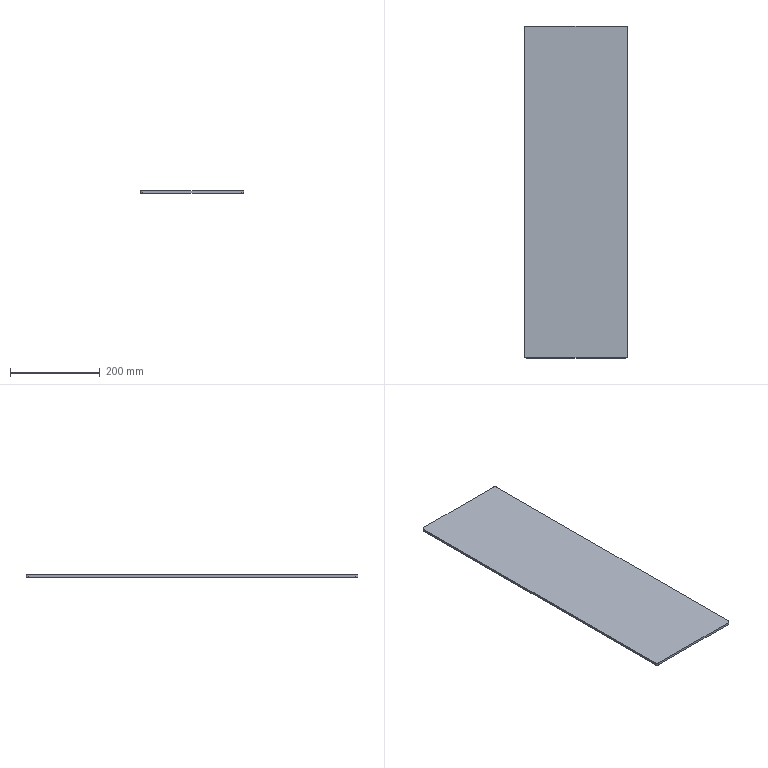Part | STEP file | 001-002-Face Plate-3 | 1 solid | 10 faces | box 230 x 740 x 5 mm | volume 850893 mm3 | plane 6 | cylinder 4 | commonest cylinder face diameters 10 x4
STEP:
#1=CARTESIAN_POINT('',(0.,0.,0.));
#2=DIRECTION('',(0.,0.,1.));
#3=DIRECTION('',(1.,0.,0.));
#4=AXIS2_PLACEMENT_3D('',#1,#2,#3);
#5=CARTESIAN_POINT('',(115.,-365.,0.));
#6=VERTEX_POINT('',#5);
#7=CARTESIAN_POINT('',(115.,365.,0.));
#8=VERTEX_POINT('',#7);
#9=CARTESIAN_POINT('',(115.,-370.,0.));
#10=DIRECTION('',(0.,1.,0.));
#11=VECTOR('',#10,1.);
#12=LINE('',#9,#11);
#13=CARTESIAN_POINT('',(115.,-370.,5.));
#14=DIRECTION('',(-1.,0.,0.));
#15=DIRECTION('',(0.,0.,1.));
#16=AXIS2_PLACEMENT_3D('',#13,#14,#15);
#17=PLANE('',#16);
#18=CARTESIAN_POINT('',(-5.,0.));
#19=DIRECTION('',(0.,1.));
#20=VECTOR('',#19,1.);
#21=LINE('',#18,#20);
#22=(GEOMETRIC_REPRESENTATION_CONTEXT(2)PARAMETRIC_REPRESENTATION_CONTEXT()REPRESENTATION_CONTEXT('',''));
#23=DEFINITIONAL_REPRESENTATION('',(#21),#22);
#24=PCURVE('',#17,#23);
#25=CARTESIAN_POINT('',(0.,0.,0.));
#26=DIRECTION('',(0.,0.,-1.));
#27=DIRECTION('',(-1.,0.,0.));
#28=AXIS2_PLACEMENT_3D('',#25,#26,#27);
#29=PLANE('',#28);
#30=CARTESIAN_POINT('',(-115.,-370.));
#31=DIRECTION('',(0.,1.));
#32=VECTOR('',#31,1.);
#33=LINE('',#30,#32);
#34=(GEOMETRIC_REPRESENTATION_CONTEXT(2)PARAMETRIC_REPRESENTATION_CONTEXT()REPRESENTATION_CONTEXT('',''));
#35=DEFINITIONAL_REPRESENTATION('',(#33),#34);
#36=PCURVE('',#29,#35);
#37=SURFACE_CURVE('',#12,(#24,#36),.PCURVE_S1.);
#38=EDGE_CURVE('',#6,#8,#37,.T.);
#39=ORIENTED_EDGE('',*,*,#38,.T.);
#40=CARTESIAN_POINT('',(115.,365.,5.));
#41=VERTEX_POINT('',#40);
#42=CARTESIAN_POINT('',(115.,365.,5.));
#43=DIRECTION('',(0.,0.,1.));
#44=VECTOR('',#43,1.);
#45=LINE('',#42,#44);
#46=CARTESIAN_POINT('',(0.,735.));
#47=DIRECTION('',(1.,0.));
#48=VECTOR('',#47,1.);
#49=LINE('',#46,#48);
#50=(GEOMETRIC_REPRESENTATION_CONTEXT(2)PARAMETRIC_REPRESENTATION_CONTEXT()REPRESENTATION_CONTEXT('',''));
#51=DEFINITIONAL_REPRESENTATION('',(#49),#50);
#52=PCURVE('',#17,#51);
#53=CARTESIAN_POINT('',(110.,365.,5.));
#54=DIRECTION('',(0.,0.,-1.));
#55=DIRECTION('',(-1.,0.,0.));
#56=AXIS2_PLACEMENT_3D('',#53,#54,#55);
#57=CYLINDRICAL_SURFACE('',#56,5.);
#58=CARTESIAN_POINT('',(3.142,0.));
#59=DIRECTION('',(0.,-1.));
#60=VECTOR('',#59,1.);
#61=LINE('',#58,#60);
#62=(GEOMETRIC_REPRESENTATION_CONTEXT(2)PARAMETRIC_REPRESENTATION_CONTEXT()REPRESENTATION_CONTEXT('',''));
#63=DEFINITIONAL_REPRESENTATION('',(#61),#62);
#64=PCURVE('',#57,#63);
#65=SURFACE_CURVE('',#45,(#52,#64),.PCURVE_S1.);
#66=EDGE_CURVE('',#8,#41,#65,.T.);
#67=ORIENTED_EDGE('',*,*,#66,.T.);
#68=CARTESIAN_POINT('',(115.,-365.,5.));
#69=VERTEX_POINT('',#68);
#70=CARTESIAN_POINT('',(115.,-370.,5.));
#71=DIRECTION('',(0.,1.,0.));
#72=VECTOR('',#71,1.);
#73=LINE('',#70,#72);
#74=CARTESIAN_POINT('',(0.,0.));
#75=DIRECTION('',(0.,1.));
#76=VECTOR('',#75,1.);
#77=LINE('',#74,#76);
#78=(GEOMETRIC_REPRESENTATION_CONTEXT(2)PARAMETRIC_REPRESENTATION_CONTEXT()REPRESENTATION_CONTEXT('',''));
#79=DEFINITIONAL_REPRESENTATION('',(#77),#78);
#80=PCURVE('',#17,#79);
#81=CARTESIAN_POINT('',(0.,0.,5.));
#82=DIRECTION('',(0.,0.,-1.));
#83=DIRECTION('',(-1.,0.,0.));
#84=AXIS2_PLACEMENT_3D('',#81,#82,#83);
#85=PLANE('',#84);
#86=CARTESIAN_POINT('',(-115.,-370.));
#87=DIRECTION('',(0.,1.));
#88=VECTOR('',#87,1.);
#89=LINE('',#86,#88);
#90=(GEOMETRIC_REPRESENTATION_CONTEXT(2)PARAMETRIC_REPRESENTATION_CONTEXT()REPRESENTATION_CONTEXT('',''));
#91=DEFINITIONAL_REPRESENTATION('',(#89),#90);
#92=PCURVE('',#85,#91);
#93=SURFACE_CURVE('',#73,(#80,#92),.PCURVE_S1.);
#94=EDGE_CURVE('',#69,#41,#93,.T.);
#95=ORIENTED_EDGE('',*,*,#94,.F.);
#96=CARTESIAN_POINT('',(115.,-365.,5.));
#97=DIRECTION('',(0.,0.,-1.));
#98=VECTOR('',#97,1.);
#99=LINE('',#96,#98);
#100=CARTESIAN_POINT('',(0.,5.));
#101=DIRECTION('',(-1.,0.));
#102=VECTOR('',#101,1.);
#103=LINE('',#100,#102);
#104=(GEOMETRIC_REPRESENTATION_CONTEXT(2)PARAMETRIC_REPRESENTATION_CONTEXT()REPRESENTATION_CONTEXT('',''));
#105=DEFINITIONAL_REPRESENTATION('',(#103),#104);
#106=PCURVE('',#17,#105);
#107=CARTESIAN_POINT('',(110.,-365.,5.));
#108=DIRECTION('',(0.,0.,-1.));
#109=DIRECTION('',(-1.,0.,0.));
#110=AXIS2_PLACEMENT_3D('',#107,#108,#109);
#111=CYLINDRICAL_SURFACE('',#110,5.);
#112=CARTESIAN_POINT('',(3.142,0.));
#113=DIRECTION('',(0.,1.));
#114=VECTOR('',#113,1.);
#115=LINE('',#112,#114);
#116=(GEOMETRIC_REPRESENTATION_CONTEXT(2)PARAMETRIC_REPRESENTATION_CONTEXT()REPRESENTATION_CONTEXT('',''));
#117=DEFINITIONAL_REPRESENTATION('',(#115),#116);
#118=PCURVE('',#111,#117);
#119=SURFACE_CURVE('',#99,(#106,#118),.PCURVE_S1.);
#120=EDGE_CURVE('',#69,#6,#119,.T.);
#121=ORIENTED_EDGE('',*,*,#120,.T.);
#122=EDGE_LOOP('',(#39,#67,#95,#121));
#123=FACE_BOUND('',#122,.T.);
#124=ADVANCED_FACE('',(#123),#17,.F.);
#125=CARTESIAN_POINT('',(110.,370.,0.));
#126=VERTEX_POINT('',#125);
#127=CARTESIAN_POINT('',(-110.,370.,0.));
#128=VERTEX_POINT('',#127);
#129=CARTESIAN_POINT('',(-115.,370.,0.));
#130=DIRECTION('',(-1.,0.,0.));
#131=VECTOR('',#130,1.);
#132=LINE('',#129,#131);
#133=CARTESIAN_POINT('',(-115.,370.,5.));
#134=DIRECTION('',(0.,-1.,0.));
#135=DIRECTION('',(0.,0.,-1.));
#136=AXIS2_PLACEMENT_3D('',#133,#134,#135);
#137=PLANE('',#136);
#138=CARTESIAN_POINT('',(5.,0.));
#139=DIRECTION('',(0.,-1.));
#140=VECTOR('',#139,1.);
#141=LINE('',#138,#140);
#142=(GEOMETRIC_REPRESENTATION_CONTEXT(2)PARAMETRIC_REPRESENTATION_CONTEXT()REPRESENTATION_CONTEXT('',''));
#143=DEFINITIONAL_REPRESENTATION('',(#141),#142);
#144=PCURVE('',#137,#143);
#145=CARTESIAN_POINT('',(115.,370.));
#146=DIRECTION('',(1.,0.));
#147=VECTOR('',#146,1.);
#148=LINE('',#145,#147);
#149=(GEOMETRIC_REPRESENTATION_CONTEXT(2)PARAMETRIC_REPRESENTATION_CONTEXT()REPRESENTATION_CONTEXT('',''));
#150=DEFINITIONAL_REPRESENTATION('',(#148),#149);
#151=PCURVE('',#29,#150);
#152=SURFACE_CURVE('',#132,(#144,#151),.PCURVE_S1.);
#153=EDGE_CURVE('',#126,#128,#152,.T.);
#154=ORIENTED_EDGE('',*,*,#153,.T.);
#155=CARTESIAN_POINT('',(-110.,370.,5.));
#156=VERTEX_POINT('',#155);
#157=CARTESIAN_POINT('',(-110.,370.,5.));
#158=DIRECTION('',(0.,0.,1.));
#159=VECTOR('',#158,1.);
#160=LINE('',#157,#159);
#161=CARTESIAN_POINT('',(0.,5.));
#162=DIRECTION('',(-1.,0.));
#163=VECTOR('',#162,1.);
#164=LINE('',#161,#163);
#165=(GEOMETRIC_REPRESENTATION_CONTEXT(2)PARAMETRIC_REPRESENTATION_CONTEXT()REPRESENTATION_CONTEXT('',''));
#166=DEFINITIONAL_REPRESENTATION('',(#164),#165);
#167=PCURVE('',#137,#166);
#168=CARTESIAN_POINT('',(-110.,365.,5.));
#169=DIRECTION('',(0.,0.,-1.));
#170=DIRECTION('',(-1.,0.,0.));
#171=AXIS2_PLACEMENT_3D('',#168,#169,#170);
#172=CYLINDRICAL_SURFACE('',#171,5.);
#173=CARTESIAN_POINT('',(1.571,0.));
#174=DIRECTION('',(0.,-1.));
#175=VECTOR('',#174,1.);
#176=LINE('',#173,#175);
#177=(GEOMETRIC_REPRESENTATION_CONTEXT(2)PARAMETRIC_REPRESENTATION_CONTEXT()REPRESENTATION_CONTEXT('',''));
#178=DEFINITIONAL_REPRESENTATION('',(#176),#177);
#179=PCURVE('',#172,#178);
#180=SURFACE_CURVE('',#160,(#167,#179),.PCURVE_S1.);
#181=EDGE_CURVE('',#128,#156,#180,.T.);
#182=ORIENTED_EDGE('',*,*,#181,.T.);
#183=CARTESIAN_POINT('',(110.,370.,5.));
#184=VERTEX_POINT('',#183);
#185=CARTESIAN_POINT('',(-115.,370.,5.));
#186=DIRECTION('',(-1.,0.,0.));
#187=VECTOR('',#186,1.);
#188=LINE('',#185,#187);
#189=CARTESIAN_POINT('',(0.,0.));
#190=DIRECTION('',(0.,-1.));
#191=VECTOR('',#190,1.);
#192=LINE('',#189,#191);
#193=(GEOMETRIC_REPRESENTATION_CONTEXT(2)PARAMETRIC_REPRESENTATION_CONTEXT()REPRESENTATION_CONTEXT('',''));
#194=DEFINITIONAL_REPRESENTATION('',(#192),#193);
#195=PCURVE('',#137,#194);
#196=CARTESIAN_POINT('',(115.,370.));
#197=DIRECTION('',(1.,0.));
#198=VECTOR('',#197,1.);
#199=LINE('',#196,#198);
#200=(GEOMETRIC_REPRESENTATION_CONTEXT(2)PARAMETRIC_REPRESENTATION_CONTEXT()REPRESENTATION_CONTEXT('',''));
#201=DEFINITIONAL_REPRESENTATION('',(#199),#200);
#202=PCURVE('',#85,#201);
#203=SURFACE_CURVE('',#188,(#195,#202),.PCURVE_S1.);
#204=EDGE_CURVE('',#184,#156,#203,.T.);
#205=ORIENTED_EDGE('',*,*,#204,.F.);
#206=CARTESIAN_POINT('',(110.,370.,5.));
#207=DIRECTION('',(0.,0.,-1.));
#208=VECTOR('',#207,1.);
#209=LINE('',#206,#208);
#210=CARTESIAN_POINT('',(0.,225.));
#211=DIRECTION('',(1.,0.));
#212=VECTOR('',#211,1.);
#213=LINE('',#210,#212);
#214=(GEOMETRIC_REPRESENTATION_CONTEXT(2)PARAMETRIC_REPRESENTATION_CONTEXT()REPRESENTATION_CONTEXT('',''));
#215=DEFINITIONAL_REPRESENTATION('',(#213),#214);
#216=PCURVE('',#137,#215);
#217=CARTESIAN_POINT('',(1.571,0.));
#218=DIRECTION('',(0.,1.));
#219=VECTOR('',#218,1.);
#220=LINE('',#217,#219);
#221=(GEOMETRIC_REPRESENTATION_CONTEXT(2)PARAMETRIC_REPRESENTATION_CONTEXT()REPRESENTATION_CONTEXT('',''));
#222=DEFINITIONAL_REPRESENTATION('',(#220),#221);
#223=PCURVE('',#57,#222);
#224=SURFACE_CURVE('',#209,(#216,#223),.PCURVE_S1.);
#225=EDGE_CURVE('',#184,#126,#224,.T.);
#226=ORIENTED_EDGE('',*,*,#225,.T.);
#227=EDGE_LOOP('',(#154,#182,#205,#226));
#228=FACE_BOUND('',#227,.T.);
#229=ADVANCED_FACE('',(#228),#137,.F.);
#230=CARTESIAN_POINT('',(-115.,365.,0.));
#231=VERTEX_POINT('',#230);
#232=CARTESIAN_POINT('',(-115.,-365.,0.));
#233=VERTEX_POINT('',#232);
#234=CARTESIAN_POINT('',(-115.,-370.,0.));
#235=DIRECTION('',(0.,-1.,0.));
#236=VECTOR('',#235,1.);
#237=LINE('',#234,#236);
#238=CARTESIAN_POINT('',(-115.,-370.,5.));
#239=DIRECTION('',(1.,0.,0.));
#240=DIRECTION('',(0.,0.,-1.));
#241=AXIS2_PLACEMENT_3D('',#238,#239,#240);
#242=PLANE('',#241);
#243=CARTESIAN_POINT('',(5.,0.));
#244=DIRECTION('',(0.,-1.));
#245=VECTOR('',#244,1.);
#246=LINE('',#243,#245);
#247=(GEOMETRIC_REPRESENTATION_CONTEXT(2)PARAMETRIC_REPRESENTATION_CONTEXT()REPRESENTATION_CONTEXT('',''));
#248=DEFINITIONAL_REPRESENTATION('',(#246),#247);
#249=PCURVE('',#242,#248);
#250=CARTESIAN_POINT('',(115.,-370.));
#251=DIRECTION('',(0.,-1.));
#252=VECTOR('',#251,1.);
#253=LINE('',#250,#252);
#254=(GEOMETRIC_REPRESENTATION_CONTEXT(2)PARAMETRIC_REPRESENTATION_CONTEXT()REPRESENTATION_CONTEXT('',''));
#255=DEFINITIONAL_REPRESENTATION('',(#253),#254);
#256=PCURVE('',#29,#255);
#257=SURFACE_CURVE('',#237,(#249,#256),.PCURVE_S1.);
#258=EDGE_CURVE('',#231,#233,#257,.T.);
#259=ORIENTED_EDGE('',*,*,#258,.T.);
#260=CARTESIAN_POINT('',(-115.,-365.,5.));
#261=VERTEX_POINT('',#260);
#262=CARTESIAN_POINT('',(-115.,-365.,5.));
#263=DIRECTION('',(0.,0.,1.));
#264=VECTOR('',#263,1.);
#265=LINE('',#262,#264);
#266=CARTESIAN_POINT('',(0.,5.));
#267=DIRECTION('',(-1.,0.));
#268=VECTOR('',#267,1.);
#269=LINE('',#266,#268);
#270=(GEOMETRIC_REPRESENTATION_CONTEXT(2)PARAMETRIC_REPRESENTATION_CONTEXT()REPRESENTATION_CONTEXT('',''));
#271=DEFINITIONAL_REPRESENTATION('',(#269),#270);
#272=PCURVE('',#242,#271);
#273=CARTESIAN_POINT('',(-110.,-365.,5.));
#274=DIRECTION('',(0.,0.,-1.));
#275=DIRECTION('',(-1.,0.,0.));
#276=AXIS2_PLACEMENT_3D('',#273,#274,#275);
#277=CYLINDRICAL_SURFACE('',#276,5.);
#278=CARTESIAN_POINT('',(6.283,0.));
#279=DIRECTION('',(0.,-1.));
#280=VECTOR('',#279,1.);
#281=LINE('',#278,#280);
#282=(GEOMETRIC_REPRESENTATION_CONTEXT(2)PARAMETRIC_REPRESENTATION_CONTEXT()REPRESENTATION_CONTEXT('',''));
#283=DEFINITIONAL_REPRESENTATION('',(#281),#282);
#284=PCURVE('',#277,#283);
#285=SURFACE_CURVE('',#265,(#272,#284),.PCURVE_S1.);
#286=EDGE_CURVE('',#233,#261,#285,.T.);
#287=ORIENTED_EDGE('',*,*,#286,.T.);
#288=CARTESIAN_POINT('',(-115.,365.,5.));
#289=VERTEX_POINT('',#288);
#290=CARTESIAN_POINT('',(-115.,-370.,5.));
#291=DIRECTION('',(0.,-1.,0.));
#292=VECTOR('',#291,1.);
#293=LINE('',#290,#292);
#294=CARTESIAN_POINT('',(0.,0.));
#295=DIRECTION('',(0.,-1.));
#296=VECTOR('',#295,1.);
#297=LINE('',#294,#296);
#298=(GEOMETRIC_REPRESENTATION_CONTEXT(2)PARAMETRIC_REPRESENTATION_CONTEXT()REPRESENTATION_CONTEXT('',''));
#299=DEFINITIONAL_REPRESENTATION('',(#297),#298);
#300=PCURVE('',#242,#299);
#301=CARTESIAN_POINT('',(115.,-370.));
#302=DIRECTION('',(0.,-1.));
#303=VECTOR('',#302,1.);
#304=LINE('',#301,#303);
#305=(GEOMETRIC_REPRESENTATION_CONTEXT(2)PARAMETRIC_REPRESENTATION_CONTEXT()REPRESENTATION_CONTEXT('',''));
#306=DEFINITIONAL_REPRESENTATION('',(#304),#305);
#307=PCURVE('',#85,#306);
#308=SURFACE_CURVE('',#293,(#300,#307),.PCURVE_S1.);
#309=EDGE_CURVE('',#289,#261,#308,.T.);
#310=ORIENTED_EDGE('',*,*,#309,.F.);
#311=CARTESIAN_POINT('',(-115.,365.,5.));
#312=DIRECTION('',(0.,0.,-1.));
#313=VECTOR('',#312,1.);
#314=LINE('',#311,#313);
#315=CARTESIAN_POINT('',(0.,735.));
#316=DIRECTION('',(1.,0.));
#317=VECTOR('',#316,1.);
#318=LINE('',#315,#317);
#319=(GEOMETRIC_REPRESENTATION_CONTEXT(2)PARAMETRIC_REPRESENTATION_CONTEXT()REPRESENTATION_CONTEXT('',''));
#320=DEFINITIONAL_REPRESENTATION('',(#318),#319);
#321=PCURVE('',#242,#320);
#322=CARTESIAN_POINT('',(0.,0.));
#323=DIRECTION('',(0.,1.));
#324=VECTOR('',#323,1.);
#325=LINE('',#322,#324);
#326=(GEOMETRIC_REPRESENTATION_CONTEXT(2)PARAMETRIC_REPRESENTATION_CONTEXT()REPRESENTATION_CONTEXT('',''));
#327=DEFINITIONAL_REPRESENTATION('',(#325),#326);
#328=PCURVE('',#172,#327);
#329=SURFACE_CURVE('',#314,(#321,#328),.PCURVE_S1.);
#330=EDGE_CURVE('',#289,#231,#329,.T.);
#331=ORIENTED_EDGE('',*,*,#330,.T.);
#332=EDGE_LOOP('',(#259,#287,#310,#331));
#333=FACE_BOUND('',#332,.T.);
#334=ADVANCED_FACE('',(#333),#242,.F.);
#335=CARTESIAN_POINT('',(-110.,-370.,5.));
#336=VERTEX_POINT('',#335);
#337=CARTESIAN_POINT('',(110.,-370.,5.));
#338=VERTEX_POINT('',#337);
#339=CARTESIAN_POINT('',(-115.,-370.,5.));
#340=DIRECTION('',(1.,0.,0.));
#341=VECTOR('',#340,1.);
#342=LINE('',#339,#341);
#343=CARTESIAN_POINT('',(-115.,-370.,5.));
#344=DIRECTION('',(0.,1.,0.));
#345=DIRECTION('',(0.,0.,1.));
#346=AXIS2_PLACEMENT_3D('',#343,#344,#345);
#347=PLANE('',#346);
#348=CARTESIAN_POINT('',(0.,0.));
#349=DIRECTION('',(0.,1.));
#350=VECTOR('',#349,1.);
#351=LINE('',#348,#350);
#352=(GEOMETRIC_REPRESENTATION_CONTEXT(2)PARAMETRIC_REPRESENTATION_CONTEXT()REPRESENTATION_CONTEXT('',''));
#353=DEFINITIONAL_REPRESENTATION('',(#351),#352);
#354=PCURVE('',#347,#353);
#355=CARTESIAN_POINT('',(115.,-370.));
#356=DIRECTION('',(-1.,0.));
#357=VECTOR('',#356,1.);
#358=LINE('',#355,#357);
#359=(GEOMETRIC_REPRESENTATION_CONTEXT(2)PARAMETRIC_REPRESENTATION_CONTEXT()REPRESENTATION_CONTEXT('',''));
#360=DEFINITIONAL_REPRESENTATION('',(#358),#359);
#361=PCURVE('',#85,#360);
#362=SURFACE_CURVE('',#342,(#354,#361),.PCURVE_S1.);
#363=EDGE_CURVE('',#336,#338,#362,.T.);
#364=ORIENTED_EDGE('',*,*,#363,.F.);
#365=CARTESIAN_POINT('',(-110.,-370.,0.));
#366=VERTEX_POINT('',#365);
#367=CARTESIAN_POINT('',(-110.,-370.,5.));
#368=DIRECTION('',(0.,0.,-1.));
#369=VECTOR('',#368,1.);
#370=LINE('',#367,#369);
#371=CARTESIAN_POINT('',(0.,5.));
#372=DIRECTION('',(-1.,0.));
#373=VECTOR('',#372,1.);
#374=LINE('',#371,#373);
#375=(GEOMETRIC_REPRESENTATION_CONTEXT(2)PARAMETRIC_REPRESENTATION_CONTEXT()REPRESENTATION_CONTEXT('',''));
#376=DEFINITIONAL_REPRESENTATION('',(#374),#375);
#377=PCURVE('',#347,#376);
#378=CARTESIAN_POINT('',(4.712,0.));
#379=DIRECTION('',(0.,1.));
#380=VECTOR('',#379,1.);
#381=LINE('',#378,#380);
#382=(GEOMETRIC_REPRESENTATION_CONTEXT(2)PARAMETRIC_REPRESENTATION_CONTEXT()REPRESENTATION_CONTEXT('',''));
#383=DEFINITIONAL_REPRESENTATION('',(#381),#382);
#384=PCURVE('',#277,#383);
#385=SURFACE_CURVE('',#370,(#377,#384),.PCURVE_S1.);
#386=EDGE_CURVE('',#336,#366,#385,.T.);
#387=ORIENTED_EDGE('',*,*,#386,.T.);
#388=CARTESIAN_POINT('',(110.,-370.,0.));
#389=VERTEX_POINT('',#388);
#390=CARTESIAN_POINT('',(-115.,-370.,0.));
#391=DIRECTION('',(1.,0.,0.));
#392=VECTOR('',#391,1.);
#393=LINE('',#390,#392);
#394=CARTESIAN_POINT('',(-5.,0.));
#395=DIRECTION('',(0.,1.));
#396=VECTOR('',#395,1.);
#397=LINE('',#394,#396);
#398=(GEOMETRIC_REPRESENTATION_CONTEXT(2)PARAMETRIC_REPRESENTATION_CONTEXT()REPRESENTATION_CONTEXT('',''));
#399=DEFINITIONAL_REPRESENTATION('',(#397),#398);
#400=PCURVE('',#347,#399);
#401=CARTESIAN_POINT('',(115.,-370.));
#402=DIRECTION('',(-1.,0.));
#403=VECTOR('',#402,1.);
#404=LINE('',#401,#403);
#405=(GEOMETRIC_REPRESENTATION_CONTEXT(2)PARAMETRIC_REPRESENTATION_CONTEXT()REPRESENTATION_CONTEXT('',''));
#406=DEFINITIONAL_REPRESENTATION('',(#404),#405);
#407=PCURVE('',#29,#406);
#408=SURFACE_CURVE('',#393,(#400,#407),.PCURVE_S1.);
#409=EDGE_CURVE('',#366,#389,#408,.T.);
#410=ORIENTED_EDGE('',*,*,#409,.T.);
#411=CARTESIAN_POINT('',(110.,-370.,5.));
#412=DIRECTION('',(0.,0.,1.));
#413=VECTOR('',#412,1.);
#414=LINE('',#411,#413);
#415=CARTESIAN_POINT('',(0.,225.));
#416=DIRECTION('',(1.,0.));
#417=VECTOR('',#416,1.);
#418=LINE('',#415,#417);
#419=(GEOMETRIC_REPRESENTATION_CONTEXT(2)PARAMETRIC_REPRESENTATION_CONTEXT()REPRESENTATION_CONTEXT('',''));
#420=DEFINITIONAL_REPRESENTATION('',(#418),#419);
#421=PCURVE('',#347,#420);
#422=CARTESIAN_POINT('',(4.712,0.));
#423=DIRECTION('',(0.,-1.));
#424=VECTOR('',#423,1.);
#425=LINE('',#422,#424);
#426=(GEOMETRIC_REPRESENTATION_CONTEXT(2)PARAMETRIC_REPRESENTATION_CONTEXT()REPRESENTATION_CONTEXT('',''));
#427=DEFINITIONAL_REPRESENTATION('',(#425),#426);
#428=PCURVE('',#111,#427);
#429=SURFACE_CURVE('',#414,(#421,#428),.PCURVE_S1.);
#430=EDGE_CURVE('',#389,#338,#429,.T.);
#431=ORIENTED_EDGE('',*,*,#430,.T.);
#432=EDGE_LOOP('',(#364,#387,#410,#431));
#433=FACE_BOUND('',#432,.T.);
#434=ADVANCED_FACE('',(#433),#347,.F.);
#435=ORIENTED_EDGE('',*,*,#309,.T.);
#436=CARTESIAN_POINT('',(-110.,-365.,5.));
#437=DIRECTION('',(0.,0.,1.));
#438=DIRECTION('',(-1.,0.,0.));
#439=AXIS2_PLACEMENT_3D('',#436,#437,#438);
#440=CIRCLE('',#439,5.);
#441=CARTESIAN_POINT('',(115.,-365.));
#442=CARTESIAN_POINT('',(115.,-373.66));
#443=CARTESIAN_POINT('',(107.5,-369.33));
#444=CARTESIAN_POINT('',(100.,-365.));
#445=CARTESIAN_POINT('',(107.5,-360.67));
#446=CARTESIAN_POINT('',(115.,-356.34));
#447=CARTESIAN_POINT('',(115.,-365.));
#448=(BOUNDED_CURVE()B_SPLINE_CURVE(2,(#441,#442,#443,#444,#445,#446,#447),.UNSPECIFIED.,.T.,.F.)B_SPLINE_CURVE_WITH_KNOTS((1,2,2,2,2,1),(-2.094,0.,2.094,4.189,6.283,8.378),.UNSPECIFIED.)CURVE()GEOMETRIC_REPRESENTATION_ITEM()RATIONAL_B_SPLINE_CURVE((1.,0.5,1.,0.5,1.,0.5,1.))REPRESENTATION_ITEM(''));
#449=(GEOMETRIC_REPRESENTATION_CONTEXT(2)PARAMETRIC_REPRESENTATION_CONTEXT()REPRESENTATION_CONTEXT('',''));
#450=DEFINITIONAL_REPRESENTATION('',(#448),#449);
#451=PCURVE('',#85,#450);
#452=CARTESIAN_POINT('',(6.283,0.));
#453=DIRECTION('',(-1.,0.));
#454=VECTOR('',#453,1.);
#455=LINE('',#452,#454);
#456=(GEOMETRIC_REPRESENTATION_CONTEXT(2)PARAMETRIC_REPRESENTATION_CONTEXT()REPRESENTATION_CONTEXT('',''));
#457=DEFINITIONAL_REPRESENTATION('',(#455),#456);
#458=PCURVE('',#277,#457);
#459=SURFACE_CURVE('',#440,(#451,#458),.PCURVE_S1.);
#460=EDGE_CURVE('',#261,#336,#459,.T.);
#461=ORIENTED_EDGE('',*,*,#460,.T.);
#462=ORIENTED_EDGE('',*,*,#363,.T.);
#463=CARTESIAN_POINT('',(110.,-365.,5.));
#464=DIRECTION('',(0.,0.,1.));
#465=DIRECTION('',(-1.,0.,0.));
#466=AXIS2_PLACEMENT_3D('',#463,#464,#465);
#467=CIRCLE('',#466,5.);
#468=CARTESIAN_POINT('',(-105.,-365.));
#469=CARTESIAN_POINT('',(-105.,-373.66));
#470=CARTESIAN_POINT('',(-112.5,-369.33));
#471=CARTESIAN_POINT('',(-120.,-365.));
#472=CARTESIAN_POINT('',(-112.5,-360.67));
#473=CARTESIAN_POINT('',(-105.,-356.34));
#474=CARTESIAN_POINT('',(-105.,-365.));
#475=(BOUNDED_CURVE()B_SPLINE_CURVE(2,(#468,#469,#470,#471,#472,#473,#474),.UNSPECIFIED.,.T.,.F.)B_SPLINE_CURVE_WITH_KNOTS((1,2,2,2,2,1),(-2.094,0.,2.094,4.189,6.283,8.378),.UNSPECIFIED.)CURVE()GEOMETRIC_REPRESENTATION_ITEM()RATIONAL_B_SPLINE_CURVE((1.,0.5,1.,0.5,1.,0.5,1.))REPRESENTATION_ITEM(''));
#476=(GEOMETRIC_REPRESENTATION_CONTEXT(2)PARAMETRIC_REPRESENTATION_CONTEXT()REPRESENTATION_CONTEXT('',''));
#477=DEFINITIONAL_REPRESENTATION('',(#475),#476);
#478=PCURVE('',#85,#477);
#479=CARTESIAN_POINT('',(6.283,0.));
#480=DIRECTION('',(-1.,0.));
#481=VECTOR('',#480,1.);
#482=LINE('',#479,#481);
#483=(GEOMETRIC_REPRESENTATION_CONTEXT(2)PARAMETRIC_REPRESENTATION_CONTEXT()REPRESENTATION_CONTEXT('',''));
#484=DEFINITIONAL_REPRESENTATION('',(#482),#483);
#485=PCURVE('',#111,#484);
#486=SURFACE_CURVE('',#467,(#478,#485),.PCURVE_S1.);
#487=EDGE_CURVE('',#338,#69,#486,.T.);
#488=ORIENTED_EDGE('',*,*,#487,.T.);
#489=ORIENTED_EDGE('',*,*,#94,.T.);
#490=CARTESIAN_POINT('',(110.,365.,5.));
#491=DIRECTION('',(0.,0.,1.));
#492=DIRECTION('',(-1.,0.,0.));
#493=AXIS2_PLACEMENT_3D('',#490,#491,#492);
#494=CIRCLE('',#493,5.);
#495=CARTESIAN_POINT('',(-105.,365.));
#496=CARTESIAN_POINT('',(-105.,356.34));
#497=CARTESIAN_POINT('',(-112.5,360.67));
#498=CARTESIAN_POINT('',(-120.,365.));
#499=CARTESIAN_POINT('',(-112.5,369.33));
#500=CARTESIAN_POINT('',(-105.,373.66));
#501=CARTESIAN_POINT('',(-105.,365.));
#502=(BOUNDED_CURVE()B_SPLINE_CURVE(2,(#495,#496,#497,#498,#499,#500,#501),.UNSPECIFIED.,.T.,.F.)B_SPLINE_CURVE_WITH_KNOTS((1,2,2,2,2,1),(-2.094,0.,2.094,4.189,6.283,8.378),.UNSPECIFIED.)CURVE()GEOMETRIC_REPRESENTATION_ITEM()RATIONAL_B_SPLINE_CURVE((1.,0.5,1.,0.5,1.,0.5,1.))REPRESENTATION_ITEM(''));
#503=(GEOMETRIC_REPRESENTATION_CONTEXT(2)PARAMETRIC_REPRESENTATION_CONTEXT()REPRESENTATION_CONTEXT('',''));
#504=DEFINITIONAL_REPRESENTATION('',(#502),#503);
#505=PCURVE('',#85,#504);
#506=CARTESIAN_POINT('',(6.283,0.));
#507=DIRECTION('',(-1.,0.));
#508=VECTOR('',#507,1.);
#509=LINE('',#506,#508);
#510=(GEOMETRIC_REPRESENTATION_CONTEXT(2)PARAMETRIC_REPRESENTATION_CONTEXT()REPRESENTATION_CONTEXT('',''));
#511=DEFINITIONAL_REPRESENTATION('',(#509),#510);
#512=PCURVE('',#57,#511);
#513=SURFACE_CURVE('',#494,(#505,#512),.PCURVE_S1.);
#514=EDGE_CURVE('',#41,#184,#513,.T.);
#515=ORIENTED_EDGE('',*,*,#514,.T.);
#516=ORIENTED_EDGE('',*,*,#204,.T.);
#517=CARTESIAN_POINT('',(-110.,365.,5.));
#518=DIRECTION('',(0.,0.,1.));
#519=DIRECTION('',(-1.,0.,0.));
#520=AXIS2_PLACEMENT_3D('',#517,#518,#519);
#521=CIRCLE('',#520,5.);
#522=CARTESIAN_POINT('',(115.,365.));
#523=CARTESIAN_POINT('',(115.,356.34));
#524=CARTESIAN_POINT('',(107.5,360.67));
#525=CARTESIAN_POINT('',(100.,365.));
#526=CARTESIAN_POINT('',(107.5,369.33));
#527=CARTESIAN_POINT('',(115.,373.66));
#528=CARTESIAN_POINT('',(115.,365.));
#529=(BOUNDED_CURVE()B_SPLINE_CURVE(2,(#522,#523,#524,#525,#526,#527,#528),.UNSPECIFIED.,.T.,.F.)B_SPLINE_CURVE_WITH_KNOTS((1,2,2,2,2,1),(-2.094,0.,2.094,4.189,6.283,8.378),.UNSPECIFIED.)CURVE()GEOMETRIC_REPRESENTATION_ITEM()RATIONAL_B_SPLINE_CURVE((1.,0.5,1.,0.5,1.,0.5,1.))REPRESENTATION_ITEM(''));
#530=(GEOMETRIC_REPRESENTATION_CONTEXT(2)PARAMETRIC_REPRESENTATION_CONTEXT()REPRESENTATION_CONTEXT('',''));
#531=DEFINITIONAL_REPRESENTATION('',(#529),#530);
#532=PCURVE('',#85,#531);
#533=CARTESIAN_POINT('',(6.283,0.));
#534=DIRECTION('',(-1.,0.));
#535=VECTOR('',#534,1.);
#536=LINE('',#533,#535);
#537=(GEOMETRIC_REPRESENTATION_CONTEXT(2)PARAMETRIC_REPRESENTATION_CONTEXT()REPRESENTATION_CONTEXT('',''));
#538=DEFINITIONAL_REPRESENTATION('',(#536),#537);
#539=PCURVE('',#172,#538);
#540=SURFACE_CURVE('',#521,(#532,#539),.PCURVE_S1.);
#541=EDGE_CURVE('',#156,#289,#540,.T.);
#542=ORIENTED_EDGE('',*,*,#541,.T.);
#543=EDGE_LOOP('',(#435,#461,#462,#488,#489,#515,#516,#542));
#544=FACE_BOUND('',#543,.T.);
#545=ADVANCED_FACE('',(#544),#85,.F.);
#546=ORIENTED_EDGE('',*,*,#409,.F.);
#547=CARTESIAN_POINT('',(-110.,-365.,0.));
#548=DIRECTION('',(0.,0.,-1.));
#549=DIRECTION('',(-1.,0.,0.));
#550=AXIS2_PLACEMENT_3D('',#547,#548,#549);
#551=CIRCLE('',#550,5.);
#552=CARTESIAN_POINT('',(110.,-365.));
#553=DIRECTION('',(1.,0.));
#554=AXIS2_PLACEMENT_2D('',#552,#553);
#555=CIRCLE('',#554,5.);
#556=(GEOMETRIC_REPRESENTATION_CONTEXT(2)PARAMETRIC_REPRESENTATION_CONTEXT()REPRESENTATION_CONTEXT('',''));
#557=DEFINITIONAL_REPRESENTATION('',(#555),#556);
#558=PCURVE('',#29,#557);
#559=CARTESIAN_POINT('',(0.,5.));
#560=DIRECTION('',(1.,0.));
#561=VECTOR('',#560,1.);
#562=LINE('',#559,#561);
#563=(GEOMETRIC_REPRESENTATION_CONTEXT(2)PARAMETRIC_REPRESENTATION_CONTEXT()REPRESENTATION_CONTEXT('',''));
#564=DEFINITIONAL_REPRESENTATION('',(#562),#563);
#565=PCURVE('',#277,#564);
#566=SURFACE_CURVE('',#551,(#558,#565),.PCURVE_S1.);
#567=EDGE_CURVE('',#366,#233,#566,.T.);
#568=ORIENTED_EDGE('',*,*,#567,.T.);
#569=ORIENTED_EDGE('',*,*,#258,.F.);
#570=CARTESIAN_POINT('',(-110.,365.,0.));
#571=DIRECTION('',(0.,0.,-1.));
#572=DIRECTION('',(-1.,0.,0.));
#573=AXIS2_PLACEMENT_3D('',#570,#571,#572);
#574=CIRCLE('',#573,5.);
#575=CARTESIAN_POINT('',(110.,365.));
#576=DIRECTION('',(1.,0.));
#577=AXIS2_PLACEMENT_2D('',#575,#576);
#578=CIRCLE('',#577,5.);
#579=(GEOMETRIC_REPRESENTATION_CONTEXT(2)PARAMETRIC_REPRESENTATION_CONTEXT()REPRESENTATION_CONTEXT('',''));
#580=DEFINITIONAL_REPRESENTATION('',(#578),#579);
#581=PCURVE('',#29,#580);
#582=CARTESIAN_POINT('',(0.,5.));
#583=DIRECTION('',(1.,0.));
#584=VECTOR('',#583,1.);
#585=LINE('',#582,#584);
#586=(GEOMETRIC_REPRESENTATION_CONTEXT(2)PARAMETRIC_REPRESENTATION_CONTEXT()REPRESENTATION_CONTEXT('',''));
#587=DEFINITIONAL_REPRESENTATION('',(#585),#586);
#588=PCURVE('',#172,#587);
#589=SURFACE_CURVE('',#574,(#581,#588),.PCURVE_S1.);
#590=EDGE_CURVE('',#231,#128,#589,.T.);
#591=ORIENTED_EDGE('',*,*,#590,.T.);
#592=ORIENTED_EDGE('',*,*,#153,.F.);
#593=CARTESIAN_POINT('',(110.,365.,0.));
#594=DIRECTION('',(0.,0.,-1.));
#595=DIRECTION('',(-1.,0.,0.));
#596=AXIS2_PLACEMENT_3D('',#593,#594,#595);
#597=CIRCLE('',#596,5.);
#598=CARTESIAN_POINT('',(-110.,365.));
#599=DIRECTION('',(1.,0.));
#600=AXIS2_PLACEMENT_2D('',#598,#599);
#601=CIRCLE('',#600,5.);
#602=(GEOMETRIC_REPRESENTATION_CONTEXT(2)PARAMETRIC_REPRESENTATION_CONTEXT()REPRESENTATION_CONTEXT('',''));
#603=DEFINITIONAL_REPRESENTATION('',(#601),#602);
#604=PCURVE('',#29,#603);
#605=CARTESIAN_POINT('',(0.,5.));
#606=DIRECTION('',(1.,0.));
#607=VECTOR('',#606,1.);
#608=LINE('',#605,#607);
#609=(GEOMETRIC_REPRESENTATION_CONTEXT(2)PARAMETRIC_REPRESENTATION_CONTEXT()REPRESENTATION_CONTEXT('',''));
#610=DEFINITIONAL_REPRESENTATION('',(#608),#609);
#611=PCURVE('',#57,#610);
#612=SURFACE_CURVE('',#597,(#604,#611),.PCURVE_S1.);
#613=EDGE_CURVE('',#126,#8,#612,.T.);
#614=ORIENTED_EDGE('',*,*,#613,.T.);
#615=ORIENTED_EDGE('',*,*,#38,.F.);
#616=CARTESIAN_POINT('',(110.,-365.,0.));
#617=DIRECTION('',(0.,0.,-1.));
#618=DIRECTION('',(-1.,0.,0.));
#619=AXIS2_PLACEMENT_3D('',#616,#617,#618);
#620=CIRCLE('',#619,5.);
#621=CARTESIAN_POINT('',(-110.,-365.));
#622=DIRECTION('',(1.,0.));
#623=AXIS2_PLACEMENT_2D('',#621,#622);
#624=CIRCLE('',#623,5.);
#625=(GEOMETRIC_REPRESENTATION_CONTEXT(2)PARAMETRIC_REPRESENTATION_CONTEXT()REPRESENTATION_CONTEXT('',''));
#626=DEFINITIONAL_REPRESENTATION('',(#624),#625);
#627=PCURVE('',#29,#626);
#628=CARTESIAN_POINT('',(0.,5.));
#629=DIRECTION('',(1.,0.));
#630=VECTOR('',#629,1.);
#631=LINE('',#628,#630);
#632=(GEOMETRIC_REPRESENTATION_CONTEXT(2)PARAMETRIC_REPRESENTATION_CONTEXT()REPRESENTATION_CONTEXT('',''));
#633=DEFINITIONAL_REPRESENTATION('',(#631),#632);
#634=PCURVE('',#111,#633);
#635=SURFACE_CURVE('',#620,(#627,#634),.PCURVE_S1.);
#636=EDGE_CURVE('',#6,#389,#635,.T.);
#637=ORIENTED_EDGE('',*,*,#636,.T.);
#638=EDGE_LOOP('',(#546,#568,#569,#591,#592,#614,#615,#637));
#639=FACE_BOUND('',#638,.T.);
#640=ADVANCED_FACE('',(#639),#29,.T.);
#641=ORIENTED_EDGE('',*,*,#460,.F.);
#642=ORIENTED_EDGE('',*,*,#286,.F.);
#643=ORIENTED_EDGE('',*,*,#567,.F.);
#644=ORIENTED_EDGE('',*,*,#386,.F.);
#645=EDGE_LOOP('',(#641,#642,#643,#644));
#646=FACE_BOUND('',#645,.T.);
#647=ADVANCED_FACE('',(#646),#277,.T.);
#648=ORIENTED_EDGE('',*,*,#541,.F.);
#649=ORIENTED_EDGE('',*,*,#181,.F.);
#650=ORIENTED_EDGE('',*,*,#590,.F.);
#651=ORIENTED_EDGE('',*,*,#330,.F.);
#652=EDGE_LOOP('',(#648,#649,#650,#651));
#653=FACE_BOUND('',#652,.T.);
#654=ADVANCED_FACE('',(#653),#172,.T.);
#655=ORIENTED_EDGE('',*,*,#514,.F.);
#656=ORIENTED_EDGE('',*,*,#66,.F.);
#657=ORIENTED_EDGE('',*,*,#613,.F.);
#658=ORIENTED_EDGE('',*,*,#225,.F.);
#659=EDGE_LOOP('',(#655,#656,#657,#658));
#660=FACE_BOUND('',#659,.T.);
#661=ADVANCED_FACE('',(#660),#57,.T.);
#662=ORIENTED_EDGE('',*,*,#487,.F.);
#663=ORIENTED_EDGE('',*,*,#430,.F.);
#664=ORIENTED_EDGE('',*,*,#636,.F.);
#665=ORIENTED_EDGE('',*,*,#120,.F.);
#666=EDGE_LOOP('',(#662,#663,#664,#665));
#667=FACE_BOUND('',#666,.T.);
#668=ADVANCED_FACE('',(#667),#111,.T.);
#669=CLOSED_SHELL('',(#124,#229,#334,#434,#545,#640,#647,#654,#661,#668));
#670=MANIFOLD_SOLID_BREP('',#669);
#671=(LENGTH_UNIT()NAMED_UNIT(*)SI_UNIT(.MILLI.,.METRE.));
#672=UNCERTAINTY_MEASURE_WITH_UNIT(LENGTH_MEASURE(0.0000001),#671,'','');
#673=(NAMED_UNIT(*)PLANE_ANGLE_UNIT()SI_UNIT($,.RADIAN.));
#674=(NAMED_UNIT(*)SI_UNIT($,.STERADIAN.)SOLID_ANGLE_UNIT());
#675=(GEOMETRIC_REPRESENTATION_CONTEXT(3)GLOBAL_UNCERTAINTY_ASSIGNED_CONTEXT((#672))GLOBAL_UNIT_ASSIGNED_CONTEXT((#671,#673,#674))REPRESENTATION_CONTEXT('',''));
#676=ADVANCED_BREP_SHAPE_REPRESENTATION('',(#4,#670),#675);